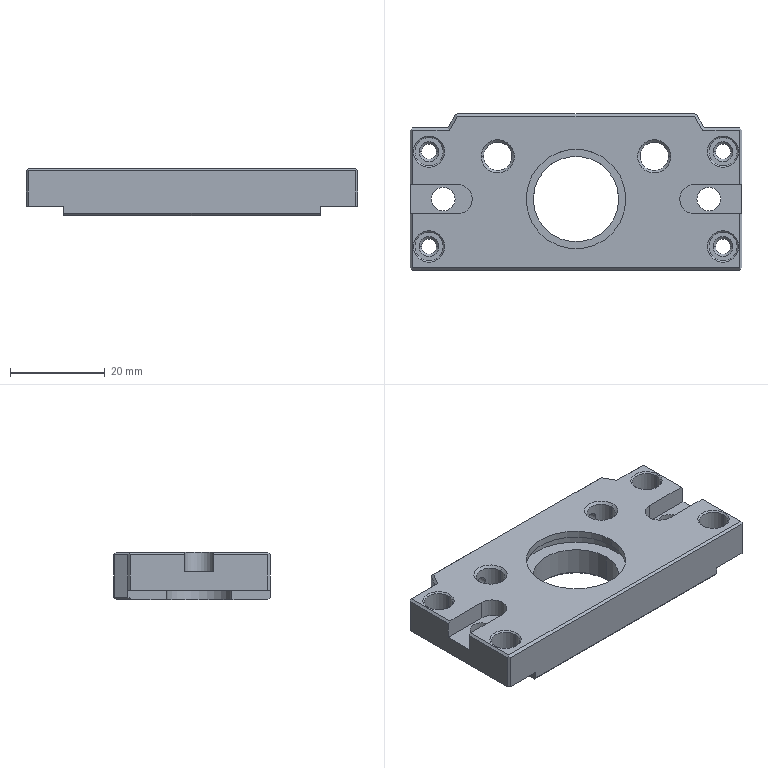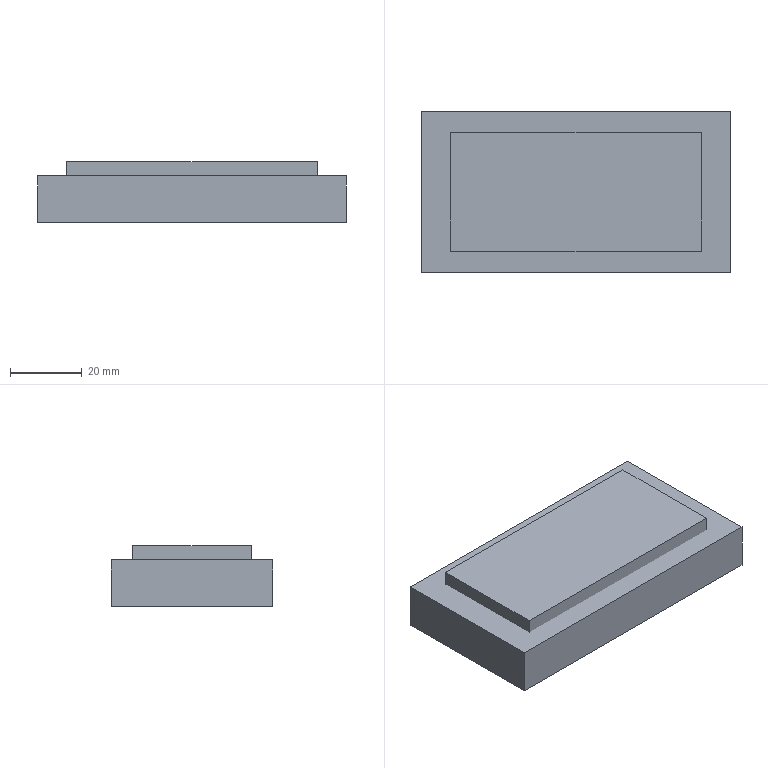CAM job | NX | 3+2 milling, drilling | part box 70 x 33 x 10 mm | stock box 86 x 45 x 17 mm
Tools:
number,name,description,diameter,corner_radius,flute_length,length,flutes
1,D50面刀,,50.0,0.0,50.0,75.0,2
11,D8,,8.0,0.0,30.0,30.0,3
7,D5精刀,,5.0,0.0,50.0,75.0,2
6,T_CUTTER,,8.0,,1.0,50.0,4
3,D10点钻,,10.0,0.0,50.0,75.0,2
4,D3.2钻头,,3.2,0.0,50.0,75.0,2
8,D5钻头,,5.0,0.0,50.0,75.0,2
2,D4C,,4.0,0.0,50.0,75.0,2
5,D5倒角刀,,5.0,0.0,50.0,75.0,2
9,D2.6,,2.6,0.0,50.0,75.0,2
10,M3,,3.0,0.0,50.0,75.0,2
Operations:
program,operation,operation_type,tool,method,geometry_group,spindle_rpm,surface_speed,feed_per_tooth,feed_cut,feed_plunge,cut_length_mm,path_length_mm,cut_time_min,machine_time_min
G54,FACE_MILLING,FaceMilling,D50面刀,MILL_FINISH,W1,4500.0,706.0,0.1111,1000.0,100.0,131.0,165.0,0.131,0.1344
G54,ADAPTIVE_MILLING,CavityMilling,D8,MILL_ROUGH,W1,5500.0,207.0,0.1818,2000.0,60.0,4189.93,4331.504,2.363,2.377
G54,PLANAR_MILL_1,PlanarMilling,D5精刀,MILL_ROUGH,W1,4500.0,70.0,0.0889,800.0,60.0,264.278,305.678,0.3439,0.3481
G54,PLANAR_MILL_2_COPY_COPY,PlanarMilling,T_CUTTER,MILL_FINISH,W1,3500.0,116.0,0.0143,200.0,100.0,59.116,101.316,0.2956,0.2998
G54,PLANAR_MILL_2,PlanarMilling,T_CUTTER,MILL_FINISH,W1,3500.0,116.0,0.0143,200.0,100.0,59.116,102.516,0.2956,0.2999
G54,PLANAR_MILL_2_COPY,PlanarMilling,T_CUTTER,MILL_FINISH,W1,3500.0,116.0,0.0143,200.0,100.0,59.116,100.116,0.2956,0.2997
G54,DRILLING_COPY,Operation,D10点钻,DRILL_METHOD,W1,1600.0,50.0,0.0625,200.0,0.0,11.0,97.061,0.055,0.0636
G54,DRILLING_COPY_COPY,Operation,D10点钻,DRILL_METHOD,W1,1600.0,50.0,0.0625,200.0,0.0,7.0,112.036,0.035,0.0455
G54,DRILLING,Operation,D10点钻,DRILL_METHOD,W1,1600.0,50.0,0.0625,200.0,0.0,21.2,193.776,0.106,0.1233
G54,DRILLING_COPY_1,Operation,D3.2钻头,DRILL_METHOD,W1,1600.0,50.0,0.0625,200.0,0.0,52.0,255.376,0.26,0.2803
G54,DRILLING_2,Operation,D5钻头,METHOD,W1,1600.0,25.0,0.0781,250.0,0.0,28.0,155.08,0.112,0.1247
G54,PLANAR_MILL,PlanarMilling,D4C,MILL_ROUGH,W1,4500.0,56.0,0.1111,1000.0,60.0,262.62,899.019,0.2893,0.3529
G54,PLANAR_PROFILE_1,PlanarMilling,D4C,MILL_FINISH,W1,4500.0,56.0,0.0444,400.0,100.0,66.472,230.592,0.1662,0.1826
G54,HOLE_MILLING_COPY,CylinderMilling,D4C,MILL_FINISH,W1,4500.0,56.0,0.0222,200.0,100.0,234.876,367.476,1.174,1.188
G54,HOLE_MILLING,CylinderMilling,D4C,MILL_FINISH,W1,4500.0,56.0,0.0222,200.0,100.0,299.906,623.106,1.5,1.532
G54,DRILLING_COPY_2,Operation,D5倒角刀,DRILL_METHOD,W1,1600.0,50.0,0.0625,200.0,0.0,32.4,239.983,0.162,0.1828
G54,PLANAR_PROFILE_COPY_1,PlanarMilling,D5倒角刀,MILL_FINISH,W1,4500.0,70.0,0.0889,800.0,100.0,222.619,262.619,0.2783,0.2823
G54,PLANAR_MILL_1_COPY_COPY,PlanarMilling,D5倒角刀,MILL_ROUGH,W1,4500.0,70.0,0.0889,800.0,60.0,62.633,103.633,0.0804,0.0845
G54,PLANAR_MILL_1_COPY_COPY_COPY,PlanarMilling,D5倒角刀,MILL_ROUGH,W1,4500.0,70.0,0.0889,800.0,60.0,50.066,99.466,0.0647,0.0697
G54,PLANAR_PROFILE_1_COPY,PlanarMilling,D5倒角刀,MILL_FINISH,W1,4500.0,70.0,0.0889,800.0,100.0,68.996,221.996,0.0862,0.1015
G54,PLANAR_MILL_1_COPY,PlanarMilling,D5精刀,MILL_FINISH,W1,4500.0,70.0,0.0444,400.0,100.0,55.839,101.239,0.1396,0.1441
G54,PLANAR_PROFILE_COPY,PlanarMilling,D5精刀,MILL_FINISH,W1,4500.0,70.0,0.0444,400.0,100.0,52.462,110.462,0.1312,0.137
G54,HOLE_MILLING_COPY_COPY,CylinderMilling,D5精刀,MILL_FINISH,W1,4500.0,70.0,0.0222,200.0,100.0,17.669,170.669,0.0883,0.1039
G54,PLANAR_PROFILE_COPY_2,PlanarMilling,D5精刀,MILL_FINISH,W1,4500.0,70.0,0.0889,800.0,100.0,227.895,285.895,0.2849,0.2907
G54,PLANAR_PROFILE,PlanarMilling,D5精刀,MILL_FINISH,W1,4500.0,70.0,0.0889,800.0,100.0,227.591,285.591,0.2845,0.2903
G55,FACE_MILLING_1,FaceMilling,D50面刀,MILL_FINISH,W2,3500.0,549.0,0.1429,1000.0,100.0,700.0,1330.5,0.7,0.763
G55,FACE_MILLING_1_COPY,FaceMilling,D50面刀,MILL_FINISH,W2,3500.0,549.0,0.0857,600.0,100.0,175.0,209.0,0.2917,0.2951
G55,FACE_MILLING_2,FaceMilling,D5精刀,MILL_ROUGH,W2,4500.0,70.0,0.1111,1000.0,60.0,645.405,1567.782,0.7053,0.7975
G55,PLANAR_PROFILE_2,PlanarMilling,D5倒角刀,MILL_FINISH,W2,4500.0,70.0,0.1111,1000.0,100.0,143.621,254.338,0.1436,0.1547
G55,PLANAR_PROFILE_2_COPY,PlanarMilling,D5倒角刀,MILL_FINISH,W2,4500.0,70.0,0.1111,1000.0,100.0,98.844,235.644,0.0988,0.1125
G55,PLANAR_PROFILE_2_COPY_COPY,PlanarMilling,D5倒角刀,MILL_FINISH,W2,4500.0,70.0,0.1111,1000.0,100.0,66.459,103.459,0.0665,0.0702
G55,PLANAR_PROFILE_2_COPY_COPY_COPY,PlanarMilling,D5倒角刀,MILL_FINISH,W2,4500.0,70.0,0.1111,1000.0,100.0,32.617,149.584,0.0326,0.0443
G55,FACE_MILLING_2_COPY,FaceMilling,D5精刀,MILL_FINISH,W2,4500.0,70.0,0.0667,600.0,100.0,319.236,773.728,0.5321,0.5775
G55,HOLE_MILLING_1,CylinderMilling,D5精刀,MILL_FINISH,W2,4500.0,70.0,0.0222,200.0,100.0,9.407,162.407,0.047,0.0623
G56,DRILLING_1,Operation,D5倒角刀,DRILL_METHOD,W3,2000.0,31.0,0.05,200.0,0.0,18.8,134.365,0.094,0.1056
G56,DRILLING_1_COPY,Operation,D2.6,DRILL_METHOD,W3,3000.0,24.0,0.0333,200.0,0.0,54.0,204.765,0.27,0.2851
G56,DRILLING_1_COPY_COPY,Operation,M3,DRILL_METHOD,W3,300.0,2.0,0.0008,0.5,0.0,36.0,168.765,72.0,72.013
G56,ZLEVEL_PROFILE,ZLevelMilling,D5精刀,MILL_FINISH,W3,5500.0,86.0,0.1364,1500.0,100.0,1828.387,1969.833,1.219,1.233
G56,FACE_MILLING_3,FaceMilling,D5精刀,MILL_FINISH,W3,4500.0,70.0,0.0667,600.0,100.0,94.0,353.866,0.1567,0.1827